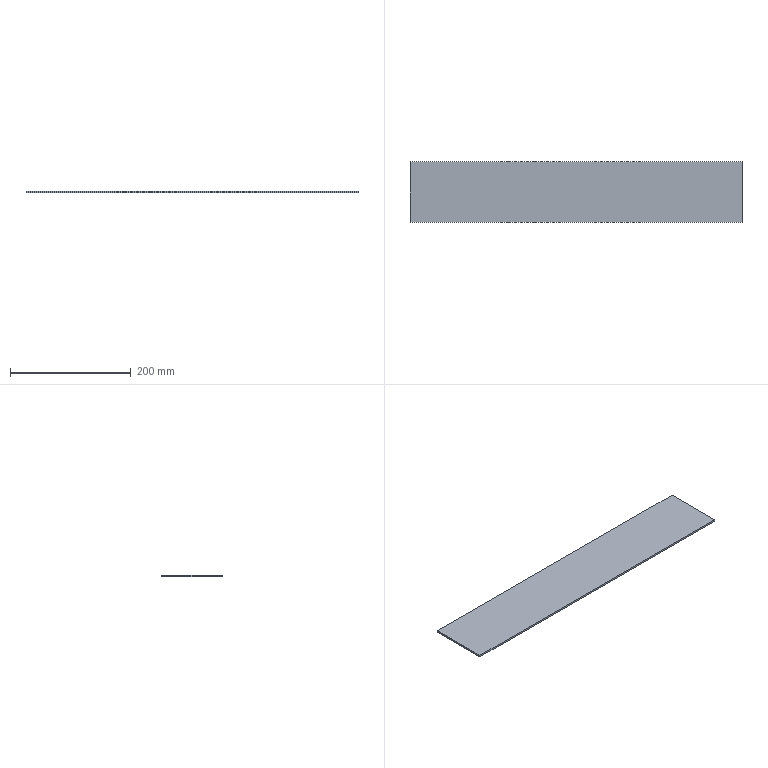Part | SolidWorks | features Extrusion 1 | 1 solid | 6 faces | box 550 x 100 x 3 mm | volume 165000 mm3 | plane 6
STEP:
#1=CARTESIAN_POINT('',(-275.,50.,0.));
#2=VERTEX_POINT('',#1);
#3=CARTESIAN_POINT('',(-275.,-50.,0.));
#4=VERTEX_POINT('',#3);
#5=CARTESIAN_POINT('',(-275.,-50.,0.));
#6=DIRECTION('',(0.,-1.,0.));
#7=VECTOR('',#6,1000.);
#8=LINE('',#5,#7);
#9=EDGE_CURVE('',#2,#4,#8,.T.);
#10=ORIENTED_EDGE('',*,*,#9,.T.);
#11=CARTESIAN_POINT('',(-275.,-50.,3.));
#12=VERTEX_POINT('',#11);
#13=CARTESIAN_POINT('',(-275.,-50.,3.));
#14=DIRECTION('',(0.,0.,-1.));
#15=VECTOR('',#14,1000.);
#16=LINE('',#13,#15);
#17=EDGE_CURVE('',#12,#4,#16,.T.);
#18=ORIENTED_EDGE('',*,*,#17,.F.);
#19=CARTESIAN_POINT('',(-275.,50.,3.));
#20=VERTEX_POINT('',#19);
#21=CARTESIAN_POINT('',(-275.,-50.,3.));
#22=DIRECTION('',(0.,-1.,0.));
#23=VECTOR('',#22,1000.);
#24=LINE('',#21,#23);
#25=EDGE_CURVE('',#20,#12,#24,.T.);
#26=ORIENTED_EDGE('',*,*,#25,.F.);
#27=CARTESIAN_POINT('',(-275.,50.,3.));
#28=DIRECTION('',(0.,0.,-1.));
#29=VECTOR('',#28,1000.);
#30=LINE('',#27,#29);
#31=EDGE_CURVE('',#20,#2,#30,.T.);
#32=ORIENTED_EDGE('',*,*,#31,.T.);
#33=EDGE_LOOP('',(#10,#18,#26,#32));
#34=FACE_OUTER_BOUND('',#33,.T.);
#35=CARTESIAN_POINT('',(-275.,-50.,3.));
#36=DIRECTION('',(1.,0.,0.));
#37=DIRECTION('',(0.,0.,-1.));
#38=AXIS2_PLACEMENT_3D('',#35,#36,#37);
#39=PLANE('',#38);
#40=ADVANCED_FACE('',(#34),#39,.F.);
#41=CARTESIAN_POINT('',(275.,-50.,0.));
#42=VERTEX_POINT('',#41);
#43=CARTESIAN_POINT('',(275.,-50.,0.));
#44=DIRECTION('',(1.,0.,0.));
#45=VECTOR('',#44,1000.);
#46=LINE('',#43,#45);
#47=EDGE_CURVE('',#4,#42,#46,.T.);
#48=ORIENTED_EDGE('',*,*,#47,.T.);
#49=CARTESIAN_POINT('',(275.,-50.,3.));
#50=VERTEX_POINT('',#49);
#51=CARTESIAN_POINT('',(275.,-50.,3.));
#52=DIRECTION('',(0.,0.,-1.));
#53=VECTOR('',#52,1000.);
#54=LINE('',#51,#53);
#55=EDGE_CURVE('',#50,#42,#54,.T.);
#56=ORIENTED_EDGE('',*,*,#55,.F.);
#57=CARTESIAN_POINT('',(275.,-50.,3.));
#58=DIRECTION('',(1.,0.,0.));
#59=VECTOR('',#58,1000.);
#60=LINE('',#57,#59);
#61=EDGE_CURVE('',#12,#50,#60,.T.);
#62=ORIENTED_EDGE('',*,*,#61,.F.);
#63=ORIENTED_EDGE('',*,*,#17,.T.);
#64=EDGE_LOOP('',(#48,#56,#62,#63));
#65=FACE_OUTER_BOUND('',#64,.T.);
#66=CARTESIAN_POINT('',(275.,-50.,3.));
#67=DIRECTION('',(0.,1.,0.));
#68=DIRECTION('',(-1.,0.,0.));
#69=AXIS2_PLACEMENT_3D('',#66,#67,#68);
#70=PLANE('',#69);
#71=ADVANCED_FACE('',(#65),#70,.F.);
#72=CARTESIAN_POINT('',(275.,50.,0.));
#73=VERTEX_POINT('',#72);
#74=CARTESIAN_POINT('',(275.,-50.,0.));
#75=DIRECTION('',(0.,1.,0.));
#76=VECTOR('',#75,1000.);
#77=LINE('',#74,#76);
#78=EDGE_CURVE('',#42,#73,#77,.T.);
#79=ORIENTED_EDGE('',*,*,#78,.T.);
#80=CARTESIAN_POINT('',(275.,50.,3.));
#81=VERTEX_POINT('',#80);
#82=CARTESIAN_POINT('',(275.,50.,3.));
#83=DIRECTION('',(0.,0.,-1.));
#84=VECTOR('',#83,1000.);
#85=LINE('',#82,#84);
#86=EDGE_CURVE('',#81,#73,#85,.T.);
#87=ORIENTED_EDGE('',*,*,#86,.F.);
#88=CARTESIAN_POINT('',(275.,-50.,3.));
#89=DIRECTION('',(0.,1.,0.));
#90=VECTOR('',#89,1000.);
#91=LINE('',#88,#90);
#92=EDGE_CURVE('',#50,#81,#91,.T.);
#93=ORIENTED_EDGE('',*,*,#92,.F.);
#94=ORIENTED_EDGE('',*,*,#55,.T.);
#95=EDGE_LOOP('',(#79,#87,#93,#94));
#96=FACE_OUTER_BOUND('',#95,.T.);
#97=CARTESIAN_POINT('',(275.,-50.,3.));
#98=DIRECTION('',(-1.,0.,0.));
#99=DIRECTION('',(0.,0.,1.));
#100=AXIS2_PLACEMENT_3D('',#97,#98,#99);
#101=PLANE('',#100);
#102=ADVANCED_FACE('',(#96),#101,.F.);
#103=CARTESIAN_POINT('',(275.,50.,0.));
#104=DIRECTION('',(-1.,0.,0.));
#105=VECTOR('',#104,1000.);
#106=LINE('',#103,#105);
#107=EDGE_CURVE('',#73,#2,#106,.T.);
#108=ORIENTED_EDGE('',*,*,#107,.T.);
#109=ORIENTED_EDGE('',*,*,#31,.F.);
#110=CARTESIAN_POINT('',(275.,50.,3.));
#111=DIRECTION('',(-1.,0.,0.));
#112=VECTOR('',#111,1000.);
#113=LINE('',#110,#112);
#114=EDGE_CURVE('',#81,#20,#113,.T.);
#115=ORIENTED_EDGE('',*,*,#114,.F.);
#116=ORIENTED_EDGE('',*,*,#86,.T.);
#117=EDGE_LOOP('',(#108,#109,#115,#116));
#118=FACE_OUTER_BOUND('',#117,.T.);
#119=CARTESIAN_POINT('',(275.,50.,3.));
#120=DIRECTION('',(0.,-1.,0.));
#121=DIRECTION('',(1.,0.,0.));
#122=AXIS2_PLACEMENT_3D('',#119,#120,#121);
#123=PLANE('',#122);
#124=ADVANCED_FACE('',(#118),#123,.F.);
#125=ORIENTED_EDGE('',*,*,#25,.T.);
#126=ORIENTED_EDGE('',*,*,#61,.T.);
#127=ORIENTED_EDGE('',*,*,#92,.T.);
#128=ORIENTED_EDGE('',*,*,#114,.T.);
#129=EDGE_LOOP('',(#125,#126,#127,#128));
#130=FACE_OUTER_BOUND('',#129,.T.);
#131=CARTESIAN_POINT('',(0.,0.,3.));
#132=DIRECTION('',(0.,0.,1.));
#133=DIRECTION('',(1.,0.,0.));
#134=AXIS2_PLACEMENT_3D('',#131,#132,#133);
#135=PLANE('',#134);
#136=ADVANCED_FACE('',(#130),#135,.T.);
#137=ORIENTED_EDGE('',*,*,#9,.F.);
#138=ORIENTED_EDGE('',*,*,#107,.F.);
#139=ORIENTED_EDGE('',*,*,#78,.F.);
#140=ORIENTED_EDGE('',*,*,#47,.F.);
#141=EDGE_LOOP('',(#137,#138,#139,#140));
#142=FACE_OUTER_BOUND('',#141,.T.);
#143=CARTESIAN_POINT('',(0.,0.,0.));
#144=DIRECTION('',(0.,0.,1.));
#145=DIRECTION('',(1.,0.,0.));
#146=AXIS2_PLACEMENT_3D('',#143,#144,#145);
#147=PLANE('',#146);
#148=ADVANCED_FACE('',(#142),#147,.F.);
#149=CLOSED_SHELL('',(#40,#71,#102,#124,#136,#148));
#150=MANIFOLD_SOLID_BREP('',#149);
#151=CARTESIAN_POINT('',(0.,0.,0.));
#152=DIRECTION('',(0.,0.,1.));
#153=DIRECTION('',(1.,0.,0.));
#154=AXIS2_PLACEMENT_3D('',#151,#152,#153);
#155=(LENGTH_UNIT()NAMED_UNIT(*)SI_UNIT(.MILLI.,.METRE.));
#156=UNCERTAINTY_MEASURE_WITH_UNIT(LENGTH_MEASURE(0.00001),#155,'','');
#157=(NAMED_UNIT(*)PLANE_ANGLE_UNIT()SI_UNIT($,.RADIAN.));
#158=(NAMED_UNIT(*)SI_UNIT($,.STERADIAN.)SOLID_ANGLE_UNIT());
#159=(GEOMETRIC_REPRESENTATION_CONTEXT(3)GLOBAL_UNCERTAINTY_ASSIGNED_CONTEXT((#156))GLOBAL_UNIT_ASSIGNED_CONTEXT((#155,#157,#158))REPRESENTATION_CONTEXT('',''));
#160=ADVANCED_BREP_SHAPE_REPRESENTATION('',(#150,#154),#159);